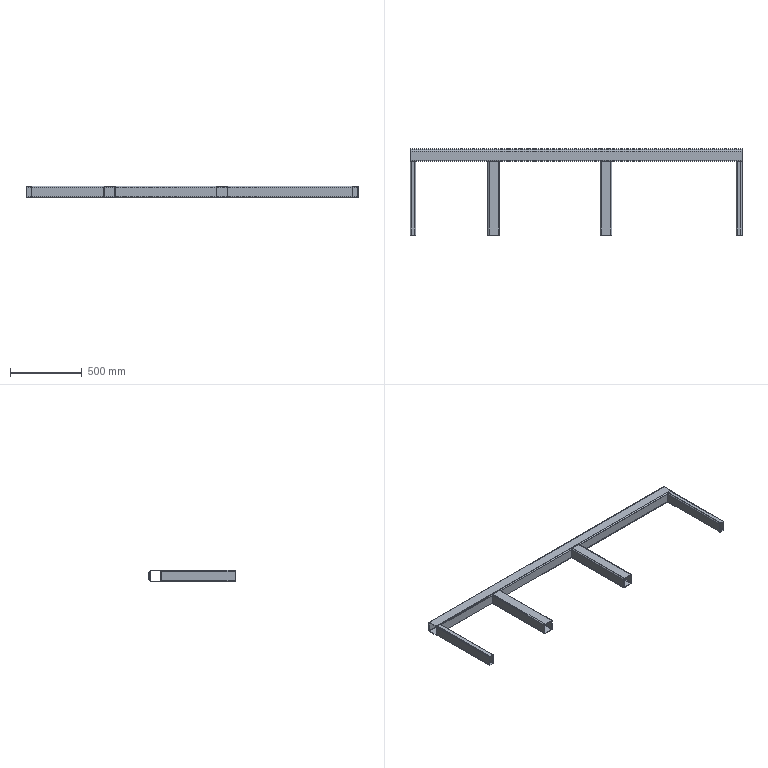Part | SolidWorks | features WeldMemberFeat 3, ICE 2, WeldCornerFeat 2, HoleWzd 1, LPattern 1, WeldmentFeature 1 | 6 solids | 196 faces | box 2320 x 602 x 80 mm | volume 5618021 mm3 | cylinder 140 | plane 56 | commonest cylinder face diameters 6.8 x100 8 x20 16 x20